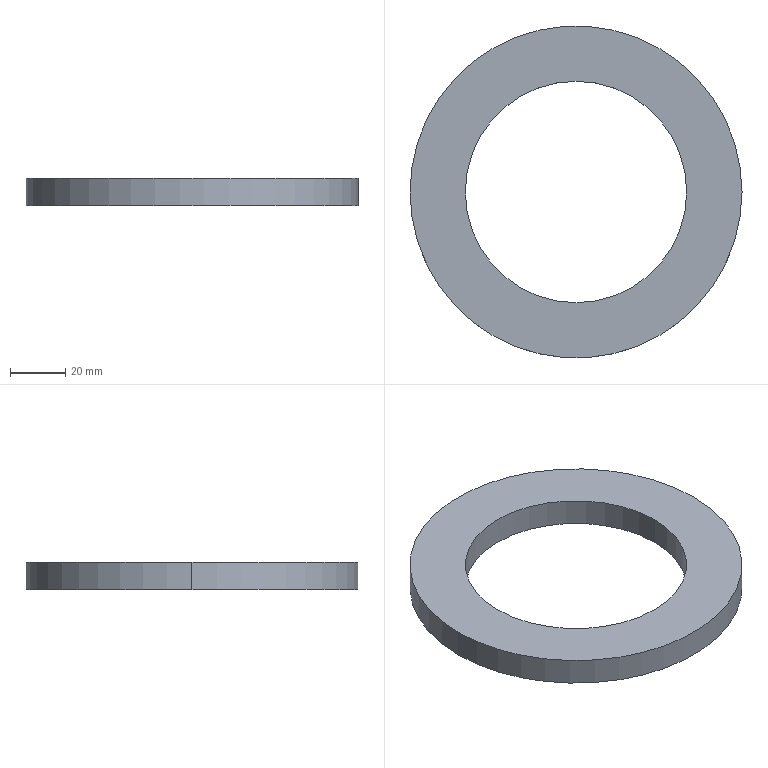Part | SolidWorks | features Extrusion 1 | 1 solid | 6 faces | box 120 x 120 x 10 mm | volume 62832 mm3 | cylinder 4 | plane 2 | commonest cylinder face diameters 80 x2 120 x2
STEP:
#1=CARTESIAN_POINT('',(-40.,0.,10.));
#2=VERTEX_POINT('',#1);
#3=CARTESIAN_POINT('',(40.,0.,10.));
#4=VERTEX_POINT('',#3);
#5=CARTESIAN_POINT('',(0.,0.,10.));
#6=DIRECTION('',(0.,0.,1.));
#7=DIRECTION('',(1.,0.,0.));
#8=AXIS2_PLACEMENT_3D('',#5,#6,#7);
#9=CIRCLE('',#8,40.);
#10=EDGE_CURVE('',#2,#4,#9,.T.);
#11=ORIENTED_EDGE('',*,*,#10,.T.);
#12=CARTESIAN_POINT('',(40.,0.,0.));
#13=VERTEX_POINT('',#12);
#14=CARTESIAN_POINT('',(40.,0.,10.));
#15=DIRECTION('',(0.,0.,-1.));
#16=VECTOR('',#15,1000.);
#17=LINE('',#14,#16);
#18=EDGE_CURVE('',#4,#13,#17,.T.);
#19=ORIENTED_EDGE('',*,*,#18,.T.);
#20=CARTESIAN_POINT('',(-40.,0.,0.));
#21=VERTEX_POINT('',#20);
#22=CARTESIAN_POINT('',(0.,0.,0.));
#23=DIRECTION('',(0.,0.,1.));
#24=DIRECTION('',(1.,0.,0.));
#25=AXIS2_PLACEMENT_3D('',#22,#23,#24);
#26=CIRCLE('',#25,40.);
#27=EDGE_CURVE('',#21,#13,#26,.T.);
#28=ORIENTED_EDGE('',*,*,#27,.F.);
#29=CARTESIAN_POINT('',(-40.,0.,10.));
#30=DIRECTION('',(0.,0.,-1.));
#31=VECTOR('',#30,1000.);
#32=LINE('',#29,#31);
#33=EDGE_CURVE('',#2,#21,#32,.T.);
#34=ORIENTED_EDGE('',*,*,#33,.F.);
#35=EDGE_LOOP('',(#11,#19,#28,#34));
#36=FACE_OUTER_BOUND('',#35,.T.);
#37=CARTESIAN_POINT('',(0.,0.,10.));
#38=DIRECTION('',(0.,0.,-1.));
#39=DIRECTION('',(-1.,0.,0.));
#40=AXIS2_PLACEMENT_3D('',#37,#38,#39);
#41=CYLINDRICAL_SURFACE('',#40,40.);
#42=ADVANCED_FACE('',(#36),#41,.F.);
#43=CARTESIAN_POINT('',(60.,0.,10.));
#44=VERTEX_POINT('',#43);
#45=CARTESIAN_POINT('',(-60.,0.,10.));
#46=VERTEX_POINT('',#45);
#47=CARTESIAN_POINT('',(0.,0.,10.));
#48=DIRECTION('',(0.,0.,1.));
#49=DIRECTION('',(1.,0.,0.));
#50=AXIS2_PLACEMENT_3D('',#47,#48,#49);
#51=CIRCLE('',#50,60.);
#52=EDGE_CURVE('',#44,#46,#51,.T.);
#53=ORIENTED_EDGE('',*,*,#52,.F.);
#54=CARTESIAN_POINT('',(60.,0.,0.));
#55=VERTEX_POINT('',#54);
#56=CARTESIAN_POINT('',(60.,0.,10.));
#57=DIRECTION('',(0.,0.,-1.));
#58=VECTOR('',#57,1000.);
#59=LINE('',#56,#58);
#60=EDGE_CURVE('',#44,#55,#59,.T.);
#61=ORIENTED_EDGE('',*,*,#60,.T.);
#62=CARTESIAN_POINT('',(-60.,0.,0.));
#63=VERTEX_POINT('',#62);
#64=CARTESIAN_POINT('',(0.,0.,0.));
#65=DIRECTION('',(0.,0.,1.));
#66=DIRECTION('',(1.,0.,0.));
#67=AXIS2_PLACEMENT_3D('',#64,#65,#66);
#68=CIRCLE('',#67,60.);
#69=EDGE_CURVE('',#55,#63,#68,.T.);
#70=ORIENTED_EDGE('',*,*,#69,.T.);
#71=CARTESIAN_POINT('',(-60.,0.,10.));
#72=DIRECTION('',(0.,0.,-1.));
#73=VECTOR('',#72,1000.);
#74=LINE('',#71,#73);
#75=EDGE_CURVE('',#46,#63,#74,.T.);
#76=ORIENTED_EDGE('',*,*,#75,.F.);
#77=EDGE_LOOP('',(#53,#61,#70,#76));
#78=FACE_OUTER_BOUND('',#77,.T.);
#79=CARTESIAN_POINT('',(0.,0.,10.));
#80=DIRECTION('',(0.,0.,-1.));
#81=DIRECTION('',(-1.,0.,0.));
#82=AXIS2_PLACEMENT_3D('',#79,#80,#81);
#83=CYLINDRICAL_SURFACE('',#82,60.);
#84=ADVANCED_FACE('',(#78),#83,.T.);
#85=CARTESIAN_POINT('',(0.,0.,10.));
#86=DIRECTION('',(0.,0.,1.));
#87=DIRECTION('',(1.,0.,0.));
#88=AXIS2_PLACEMENT_3D('',#85,#86,#87);
#89=CIRCLE('',#88,60.);
#90=EDGE_CURVE('',#46,#44,#89,.T.);
#91=ORIENTED_EDGE('',*,*,#90,.T.);
#92=ORIENTED_EDGE('',*,*,#52,.T.);
#93=EDGE_LOOP('',(#91,#92));
#94=FACE_OUTER_BOUND('',#93,.T.);
#95=ORIENTED_EDGE('',*,*,#10,.F.);
#96=CARTESIAN_POINT('',(0.,0.,10.));
#97=DIRECTION('',(0.,0.,1.));
#98=DIRECTION('',(1.,0.,0.));
#99=AXIS2_PLACEMENT_3D('',#96,#97,#98);
#100=CIRCLE('',#99,40.);
#101=EDGE_CURVE('',#4,#2,#100,.T.);
#102=ORIENTED_EDGE('',*,*,#101,.F.);
#103=EDGE_LOOP('',(#95,#102));
#104=FACE_BOUND('',#103,.T.);
#105=CARTESIAN_POINT('',(0.,0.,10.));
#106=DIRECTION('',(0.,0.,1.));
#107=DIRECTION('',(1.,0.,0.));
#108=AXIS2_PLACEMENT_3D('',#105,#106,#107);
#109=PLANE('',#108);
#110=ADVANCED_FACE('',(#94,#104),#109,.T.);
#111=CARTESIAN_POINT('',(0.,0.,0.));
#112=DIRECTION('',(0.,0.,1.));
#113=DIRECTION('',(1.,0.,0.));
#114=AXIS2_PLACEMENT_3D('',#111,#112,#113);
#115=CIRCLE('',#114,60.);
#116=EDGE_CURVE('',#63,#55,#115,.T.);
#117=ORIENTED_EDGE('',*,*,#116,.F.);
#118=ORIENTED_EDGE('',*,*,#69,.F.);
#119=EDGE_LOOP('',(#117,#118));
#120=FACE_OUTER_BOUND('',#119,.T.);
#121=ORIENTED_EDGE('',*,*,#27,.T.);
#122=CARTESIAN_POINT('',(0.,0.,0.));
#123=DIRECTION('',(0.,0.,1.));
#124=DIRECTION('',(1.,0.,0.));
#125=AXIS2_PLACEMENT_3D('',#122,#123,#124);
#126=CIRCLE('',#125,40.);
#127=EDGE_CURVE('',#13,#21,#126,.T.);
#128=ORIENTED_EDGE('',*,*,#127,.T.);
#129=EDGE_LOOP('',(#121,#128));
#130=FACE_BOUND('',#129,.T.);
#131=CARTESIAN_POINT('',(0.,0.,0.));
#132=DIRECTION('',(0.,0.,1.));
#133=DIRECTION('',(1.,0.,0.));
#134=AXIS2_PLACEMENT_3D('',#131,#132,#133);
#135=PLANE('',#134);
#136=ADVANCED_FACE('',(#120,#130),#135,.F.);
#137=ORIENTED_EDGE('',*,*,#60,.F.);
#138=ORIENTED_EDGE('',*,*,#90,.F.);
#139=ORIENTED_EDGE('',*,*,#75,.T.);
#140=ORIENTED_EDGE('',*,*,#116,.T.);
#141=EDGE_LOOP('',(#137,#138,#139,#140));
#142=FACE_OUTER_BOUND('',#141,.T.);
#143=CARTESIAN_POINT('',(0.,0.,10.));
#144=DIRECTION('',(0.,0.,-1.));
#145=DIRECTION('',(-1.,0.,0.));
#146=AXIS2_PLACEMENT_3D('',#143,#144,#145);
#147=CYLINDRICAL_SURFACE('',#146,60.);
#148=ADVANCED_FACE('',(#142),#147,.T.);
#149=ORIENTED_EDGE('',*,*,#18,.F.);
#150=ORIENTED_EDGE('',*,*,#101,.T.);
#151=ORIENTED_EDGE('',*,*,#33,.T.);
#152=ORIENTED_EDGE('',*,*,#127,.F.);
#153=EDGE_LOOP('',(#149,#150,#151,#152));
#154=FACE_OUTER_BOUND('',#153,.T.);
#155=CARTESIAN_POINT('',(0.,0.,10.));
#156=DIRECTION('',(0.,0.,-1.));
#157=DIRECTION('',(-1.,0.,0.));
#158=AXIS2_PLACEMENT_3D('',#155,#156,#157);
#159=CYLINDRICAL_SURFACE('',#158,40.);
#160=ADVANCED_FACE('',(#154),#159,.F.);
#161=CLOSED_SHELL('',(#42,#84,#110,#136,#148,#160));
#162=MANIFOLD_SOLID_BREP('',#161);
#163=CARTESIAN_POINT('',(0.,0.,0.));
#164=DIRECTION('',(0.,0.,1.));
#165=DIRECTION('',(1.,0.,0.));
#166=AXIS2_PLACEMENT_3D('',#163,#164,#165);
#167=(LENGTH_UNIT()NAMED_UNIT(*)SI_UNIT(.MILLI.,.METRE.));
#168=UNCERTAINTY_MEASURE_WITH_UNIT(LENGTH_MEASURE(0.00001),#167,'','');
#169=(NAMED_UNIT(*)PLANE_ANGLE_UNIT()SI_UNIT($,.RADIAN.));
#170=(NAMED_UNIT(*)SI_UNIT($,.STERADIAN.)SOLID_ANGLE_UNIT());
#171=(GEOMETRIC_REPRESENTATION_CONTEXT(3)GLOBAL_UNCERTAINTY_ASSIGNED_CONTEXT((#168))GLOBAL_UNIT_ASSIGNED_CONTEXT((#167,#169,#170))REPRESENTATION_CONTEXT('',''));
#172=ADVANCED_BREP_SHAPE_REPRESENTATION('',(#162,#166),#171);